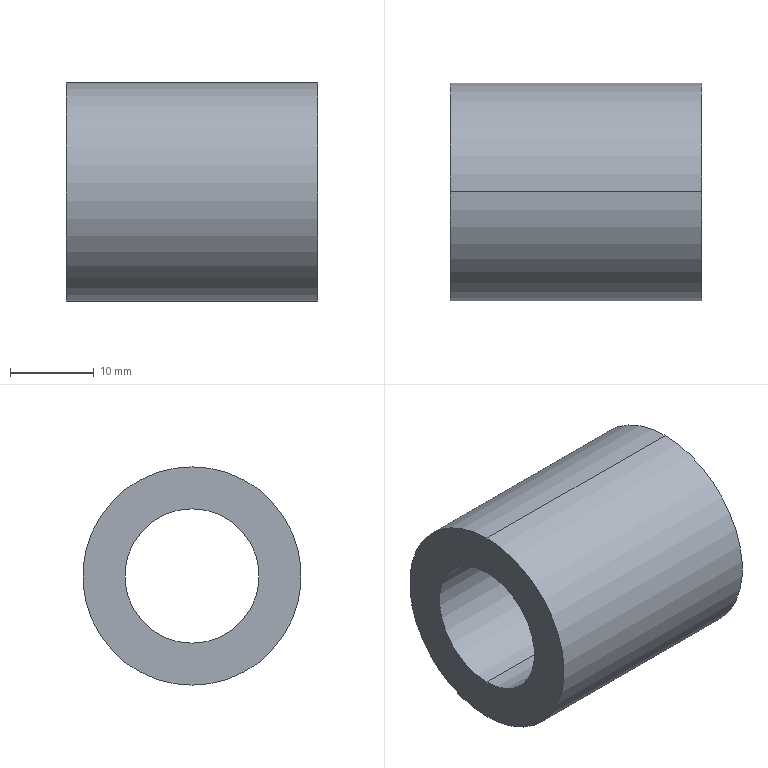Part | SolidWorks | features BaseBody 1 | 1 solid | 6 faces | box 30 x 26 x 26 mm | volume 9896 mm3 | cylinder 4 | plane 2 | commonest cylinder face diameters 16 x2 26 x2
STEP:
#1=CARTESIAN_POINT('',(-104.,-23.,-124.));
#2=VERTEX_POINT('',#1);
#3=CARTESIAN_POINT('',(-104.,-23.,-150.));
#4=VERTEX_POINT('',#3);
#5=CARTESIAN_POINT('',(-104.,-23.,-137.));
#6=DIRECTION('',(-1.,0.,0.));
#7=DIRECTION('',(0.,0.,1.));
#8=AXIS2_PLACEMENT_3D('',#5,#6,#7);
#9=CIRCLE('',#8,13.);
#10=EDGE_CURVE('',#2,#4,#9,.T.);
#11=ORIENTED_EDGE('',*,*,#10,.T.);
#12=CARTESIAN_POINT('',(-134.,-23.,-150.));
#13=VERTEX_POINT('',#12);
#14=CARTESIAN_POINT('',(-104.,-23.,-150.));
#15=DIRECTION('',(-1.,0.,0.));
#16=VECTOR('',#15,1000.);
#17=LINE('',#14,#16);
#18=EDGE_CURVE('',#4,#13,#17,.T.);
#19=ORIENTED_EDGE('',*,*,#18,.T.);
#20=CARTESIAN_POINT('',(-134.,-23.,-124.));
#21=VERTEX_POINT('',#20);
#22=CARTESIAN_POINT('',(-134.,-23.,-137.));
#23=DIRECTION('',(1.,0.,0.));
#24=DIRECTION('',(0.,0.,1.));
#25=AXIS2_PLACEMENT_3D('',#22,#23,#24);
#26=CIRCLE('',#25,13.);
#27=EDGE_CURVE('',#13,#21,#26,.T.);
#28=ORIENTED_EDGE('',*,*,#27,.T.);
#29=CARTESIAN_POINT('',(-104.,-23.,-124.));
#30=DIRECTION('',(-1.,0.,0.));
#31=VECTOR('',#30,1000.);
#32=LINE('',#29,#31);
#33=EDGE_CURVE('',#2,#21,#32,.T.);
#34=ORIENTED_EDGE('',*,*,#33,.F.);
#35=EDGE_LOOP('',(#11,#19,#28,#34));
#36=FACE_OUTER_BOUND('',#35,.T.);
#37=CARTESIAN_POINT('',(-104.,-23.,-137.));
#38=DIRECTION('',(-1.,0.,0.));
#39=DIRECTION('',(0.,0.,1.));
#40=AXIS2_PLACEMENT_3D('',#37,#38,#39);
#41=CYLINDRICAL_SURFACE('',#40,13.);
#42=ADVANCED_FACE('',(#36),#41,.T.);
#43=CARTESIAN_POINT('',(-104.,-23.,-145.));
#44=VERTEX_POINT('',#43);
#45=CARTESIAN_POINT('',(-104.,-23.,-129.));
#46=VERTEX_POINT('',#45);
#47=CARTESIAN_POINT('',(-104.,-23.,-137.));
#48=DIRECTION('',(-1.,0.,0.));
#49=DIRECTION('',(0.,0.,1.));
#50=AXIS2_PLACEMENT_3D('',#47,#48,#49);
#51=CIRCLE('',#50,8.);
#52=EDGE_CURVE('',#44,#46,#51,.T.);
#53=ORIENTED_EDGE('',*,*,#52,.F.);
#54=CARTESIAN_POINT('',(-134.,-23.,-145.));
#55=VERTEX_POINT('',#54);
#56=CARTESIAN_POINT('',(-104.,-23.,-145.));
#57=DIRECTION('',(-1.,0.,0.));
#58=VECTOR('',#57,1000.);
#59=LINE('',#56,#58);
#60=EDGE_CURVE('',#44,#55,#59,.T.);
#61=ORIENTED_EDGE('',*,*,#60,.T.);
#62=CARTESIAN_POINT('',(-134.,-23.,-129.));
#63=VERTEX_POINT('',#62);
#64=CARTESIAN_POINT('',(-134.,-23.,-137.));
#65=DIRECTION('',(-1.,0.,0.));
#66=DIRECTION('',(0.,0.,1.));
#67=AXIS2_PLACEMENT_3D('',#64,#65,#66);
#68=CIRCLE('',#67,8.);
#69=EDGE_CURVE('',#55,#63,#68,.T.);
#70=ORIENTED_EDGE('',*,*,#69,.T.);
#71=CARTESIAN_POINT('',(-104.,-23.,-129.));
#72=DIRECTION('',(-1.,0.,0.));
#73=VECTOR('',#72,1000.);
#74=LINE('',#71,#73);
#75=EDGE_CURVE('',#46,#63,#74,.T.);
#76=ORIENTED_EDGE('',*,*,#75,.F.);
#77=EDGE_LOOP('',(#53,#61,#70,#76));
#78=FACE_OUTER_BOUND('',#77,.T.);
#79=CARTESIAN_POINT('',(-104.,-23.,-137.));
#80=DIRECTION('',(-1.,0.,0.));
#81=DIRECTION('',(0.,0.,1.));
#82=AXIS2_PLACEMENT_3D('',#79,#80,#81);
#83=CYLINDRICAL_SURFACE('',#82,8.);
#84=ADVANCED_FACE('',(#78),#83,.F.);
#85=ORIENTED_EDGE('',*,*,#18,.F.);
#86=CARTESIAN_POINT('',(-104.,-23.,-137.));
#87=DIRECTION('',(-1.,0.,0.));
#88=DIRECTION('',(0.,0.,1.));
#89=AXIS2_PLACEMENT_3D('',#86,#87,#88);
#90=CIRCLE('',#89,13.);
#91=EDGE_CURVE('',#4,#2,#90,.T.);
#92=ORIENTED_EDGE('',*,*,#91,.T.);
#93=ORIENTED_EDGE('',*,*,#33,.T.);
#94=CARTESIAN_POINT('',(-134.,-23.,-137.));
#95=DIRECTION('',(1.,0.,0.));
#96=DIRECTION('',(0.,0.,1.));
#97=AXIS2_PLACEMENT_3D('',#94,#95,#96);
#98=CIRCLE('',#97,13.);
#99=EDGE_CURVE('',#21,#13,#98,.T.);
#100=ORIENTED_EDGE('',*,*,#99,.T.);
#101=EDGE_LOOP('',(#85,#92,#93,#100));
#102=FACE_OUTER_BOUND('',#101,.T.);
#103=CARTESIAN_POINT('',(-104.,-23.,-137.));
#104=DIRECTION('',(-1.,0.,0.));
#105=DIRECTION('',(0.,0.,1.));
#106=AXIS2_PLACEMENT_3D('',#103,#104,#105);
#107=CYLINDRICAL_SURFACE('',#106,13.);
#108=ADVANCED_FACE('',(#102),#107,.T.);
#109=CARTESIAN_POINT('',(-104.,-23.,-137.));
#110=DIRECTION('',(-1.,0.,0.));
#111=DIRECTION('',(0.,0.,1.));
#112=AXIS2_PLACEMENT_3D('',#109,#110,#111);
#113=CIRCLE('',#112,8.);
#114=EDGE_CURVE('',#46,#44,#113,.T.);
#115=ORIENTED_EDGE('',*,*,#114,.T.);
#116=ORIENTED_EDGE('',*,*,#52,.T.);
#117=EDGE_LOOP('',(#115,#116));
#118=FACE_BOUND('',#117,.T.);
#119=ORIENTED_EDGE('',*,*,#10,.F.);
#120=ORIENTED_EDGE('',*,*,#91,.F.);
#121=EDGE_LOOP('',(#119,#120));
#122=FACE_OUTER_BOUND('',#121,.T.);
#123=CARTESIAN_POINT('',(-104.,-23.,-137.));
#124=DIRECTION('',(1.,0.,0.));
#125=DIRECTION('',(0.,0.,-1.));
#126=AXIS2_PLACEMENT_3D('',#123,#124,#125);
#127=PLANE('',#126);
#128=ADVANCED_FACE('',(#118,#122),#127,.T.);
#129=CARTESIAN_POINT('',(-134.,-23.,-137.));
#130=DIRECTION('',(-1.,0.,0.));
#131=DIRECTION('',(0.,0.,1.));
#132=AXIS2_PLACEMENT_3D('',#129,#130,#131);
#133=CIRCLE('',#132,8.);
#134=EDGE_CURVE('',#63,#55,#133,.T.);
#135=ORIENTED_EDGE('',*,*,#134,.F.);
#136=ORIENTED_EDGE('',*,*,#69,.F.);
#137=EDGE_LOOP('',(#135,#136));
#138=FACE_BOUND('',#137,.T.);
#139=ORIENTED_EDGE('',*,*,#99,.F.);
#140=ORIENTED_EDGE('',*,*,#27,.F.);
#141=EDGE_LOOP('',(#139,#140));
#142=FACE_OUTER_BOUND('',#141,.T.);
#143=CARTESIAN_POINT('',(-134.,-23.,-137.));
#144=DIRECTION('',(1.,0.,0.));
#145=DIRECTION('',(0.,0.,-1.));
#146=AXIS2_PLACEMENT_3D('',#143,#144,#145);
#147=PLANE('',#146);
#148=ADVANCED_FACE('',(#138,#142),#147,.F.);
#149=ORIENTED_EDGE('',*,*,#60,.F.);
#150=ORIENTED_EDGE('',*,*,#114,.F.);
#151=ORIENTED_EDGE('',*,*,#75,.T.);
#152=ORIENTED_EDGE('',*,*,#134,.T.);
#153=EDGE_LOOP('',(#149,#150,#151,#152));
#154=FACE_OUTER_BOUND('',#153,.T.);
#155=CARTESIAN_POINT('',(-104.,-23.,-137.));
#156=DIRECTION('',(-1.,0.,0.));
#157=DIRECTION('',(0.,0.,1.));
#158=AXIS2_PLACEMENT_3D('',#155,#156,#157);
#159=CYLINDRICAL_SURFACE('',#158,8.);
#160=ADVANCED_FACE('',(#154),#159,.F.);
#161=CLOSED_SHELL('',(#42,#84,#108,#128,#148,#160));
#162=MANIFOLD_SOLID_BREP('',#161);
#163=CARTESIAN_POINT('',(0.,0.,0.));
#164=DIRECTION('',(0.,0.,1.));
#165=DIRECTION('',(1.,0.,0.));
#166=AXIS2_PLACEMENT_3D('',#163,#164,#165);
#167=(LENGTH_UNIT()NAMED_UNIT(*)SI_UNIT(.MILLI.,.METRE.));
#168=UNCERTAINTY_MEASURE_WITH_UNIT(LENGTH_MEASURE(0.00001),#167,'','');
#169=(NAMED_UNIT(*)PLANE_ANGLE_UNIT()SI_UNIT($,.RADIAN.));
#170=(NAMED_UNIT(*)SI_UNIT($,.STERADIAN.)SOLID_ANGLE_UNIT());
#171=(GEOMETRIC_REPRESENTATION_CONTEXT(3)GLOBAL_UNCERTAINTY_ASSIGNED_CONTEXT((#168))GLOBAL_UNIT_ASSIGNED_CONTEXT((#167,#169,#170))REPRESENTATION_CONTEXT('',''));
#172=ADVANCED_BREP_SHAPE_REPRESENTATION('',(#162,#166),#171);